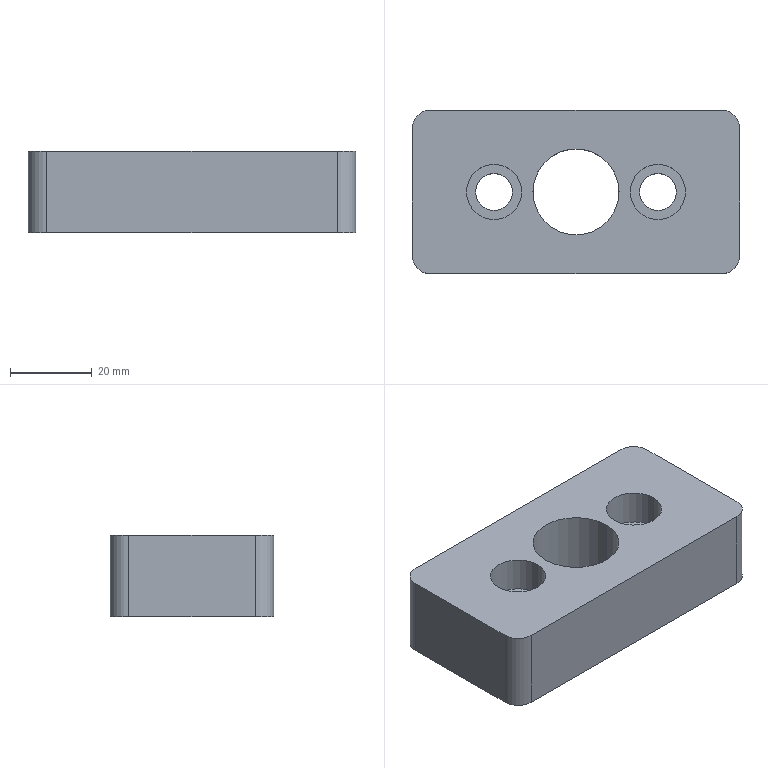Part | STEP file | Foot mounting block | 1 solid | 22 faces | box 80 x 40 x 20 mm | volume 52813 mm3 | cylinder 14 | plane 8 | commonest cylinder face diameters 9 x8 13.5 x4 21 x2